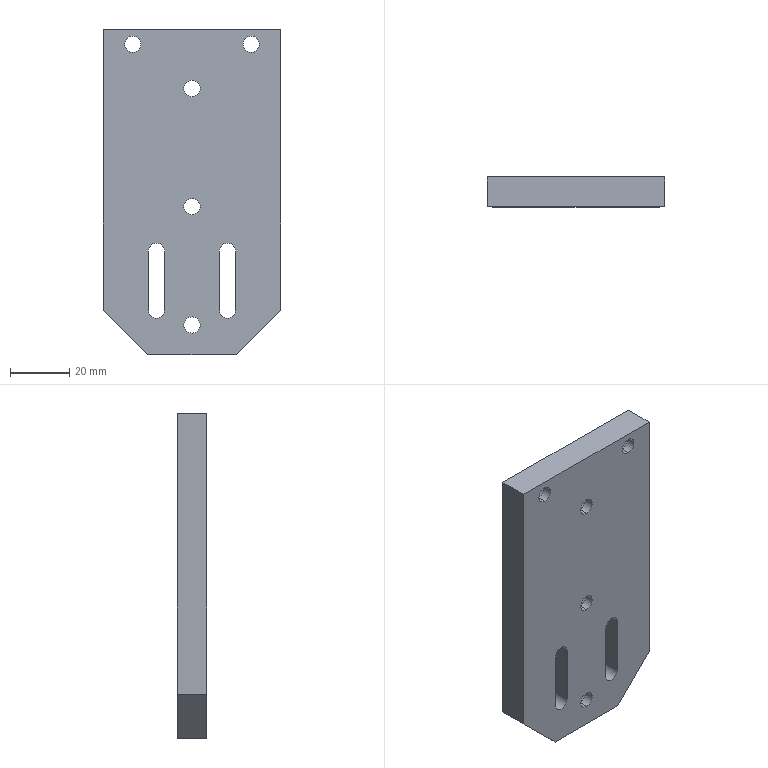Part | STEP file | B1-015 | 1 solid | 43 faces | box 60 x 10 x 110 mm | volume 58492 mm3 | cylinder 26 | plane 17 | commonest cylinder face diameters 5.5 x16 9 x10